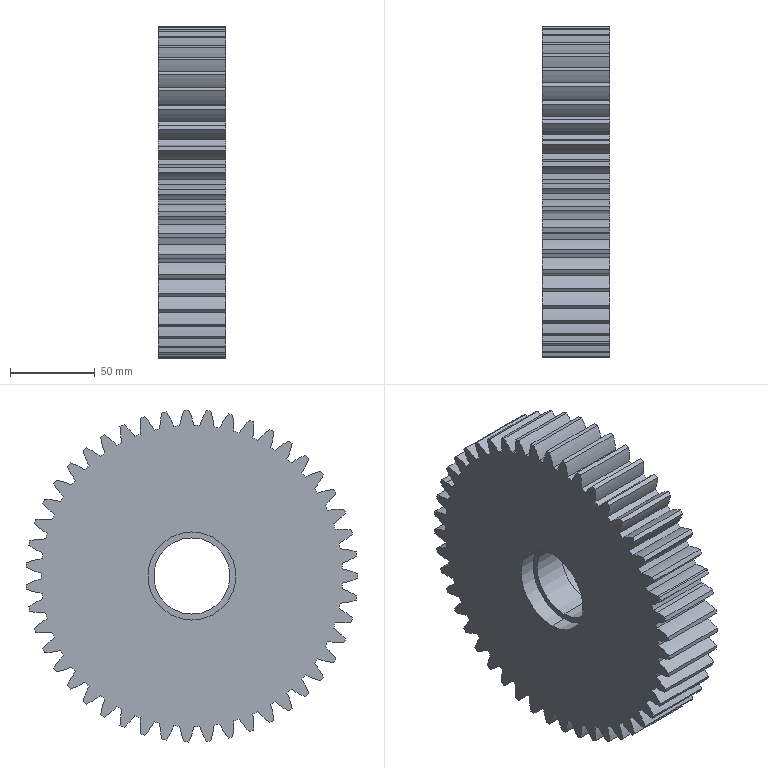Part | SolidWorks | features ICE 1, MBimport 1, MirrorPattern 1 | 1 solid | 202 faces | box 40 x 195.86 x 195.96 mm | volume 1021881 mm3 | cylinder 198 | plane 4 | commonest cylinder face diameters 75.2 x98 177.998 x47 196 x47 52 x4 45 x2